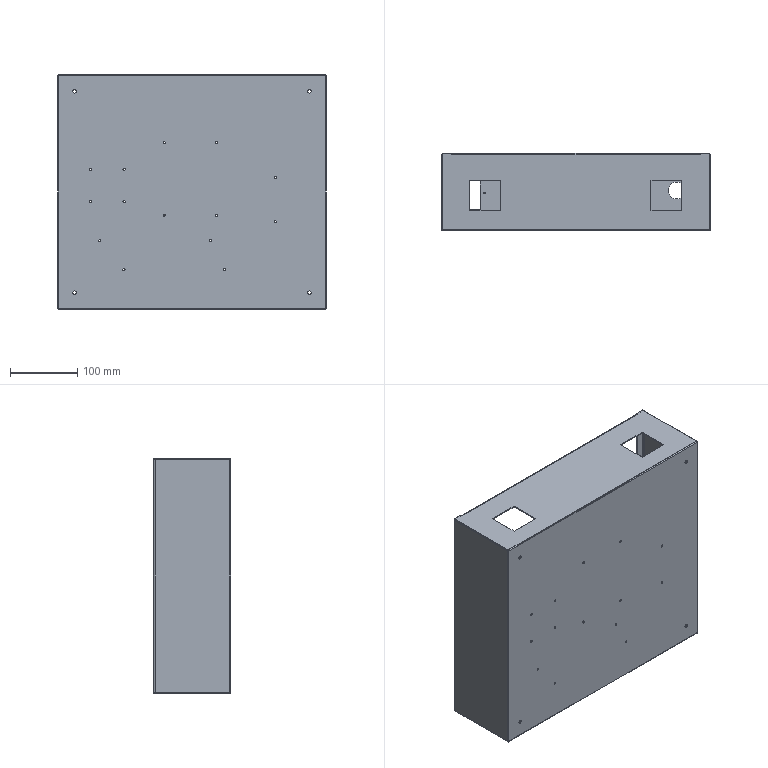Part | STEP file | Electrical box 400-350 | 1 solid | 146 faces | box 400 x 115 x 350 mm | volume 480452 mm3 | plane 86 | cylinder 60 | commonest cylinder face diameters 3.3 x28 5 x12 2.5 x8 2 x4 3 x4 16 x2